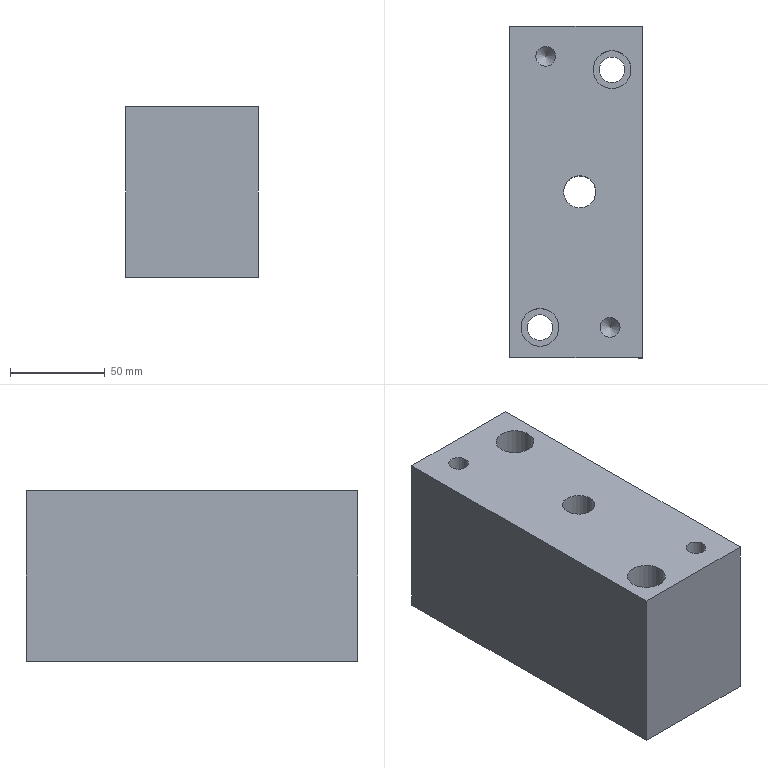Part | STEP file | lll_id4278_x_t | 1 solid | 17 faces | box 70 x 175 x 90 mm | volume 1031472 mm3 | plane 8 | cylinder 7 | cone 2 | commonest cylinder face diameters 10.506 x2 13.509 x2 20.008 x2 17 x1
STEP:
#1=CARTESIAN_POINT('',(3003.,-87.5,-90.));
#2=VERTEX_POINT('',#1);
#3=CARTESIAN_POINT('',(2933.,-87.5,-90.));
#4=VERTEX_POINT('',#3);
#5=CARTESIAN_POINT('',(13471.883,-87.5,-90.));
#6=DIRECTION('',(-1.,0.,0.));
#7=VECTOR('',#6,1.);
#8=LINE('',#5,#7);
#9=EDGE_CURVE('',#2,#4,#8,.T.);
#10=ORIENTED_EDGE('',*,*,#9,.F.);
#11=CARTESIAN_POINT('',(3003.,-87.5,0.));
#12=VERTEX_POINT('',#11);
#13=CARTESIAN_POINT('',(3003.,-87.5,0.));
#14=DIRECTION('',(0.,0.,1.));
#15=VECTOR('',#14,1.);
#16=LINE('',#13,#15);
#17=EDGE_CURVE('',#2,#12,#16,.T.);
#18=ORIENTED_EDGE('',*,*,#17,.T.);
#19=CARTESIAN_POINT('',(2933.,-87.5,0.));
#20=VERTEX_POINT('',#19);
#21=CARTESIAN_POINT('',(13471.883,-87.5,0.));
#22=DIRECTION('',(1.,0.,0.));
#23=VECTOR('',#22,1.);
#24=LINE('',#21,#23);
#25=EDGE_CURVE('',#20,#12,#24,.T.);
#26=ORIENTED_EDGE('',*,*,#25,.F.);
#27=CARTESIAN_POINT('',(2933.,-87.5,0.));
#28=DIRECTION('',(0.,0.,-1.));
#29=VECTOR('',#28,1.);
#30=LINE('',#27,#29);
#31=EDGE_CURVE('',#20,#4,#30,.T.);
#32=ORIENTED_EDGE('',*,*,#31,.T.);
#33=EDGE_LOOP('',(#10,#18,#26,#32));
#34=FACE_OUTER_BOUND('',#33,.T.);
#35=CARTESIAN_POINT('',(13471.883,-87.5,0.));
#36=DIRECTION('',(0.,1.,0.));
#37=DIRECTION('',(1.,0.,0.));
#38=AXIS2_PLACEMENT_3D('',#35,#36,#37);
#39=PLANE('',#38);
#40=ADVANCED_FACE('',(#34),#39,.F.);
#41=CARTESIAN_POINT('',(2933.,87.5,-90.));
#42=VERTEX_POINT('',#41);
#43=CARTESIAN_POINT('',(2933.,38.,-90.));
#44=DIRECTION('',(0.,-1.,0.));
#45=VECTOR('',#44,1.);
#46=LINE('',#43,#45);
#47=EDGE_CURVE('',#42,#4,#46,.T.);
#48=ORIENTED_EDGE('',*,*,#47,.T.);
#49=ORIENTED_EDGE('',*,*,#31,.F.);
#50=CARTESIAN_POINT('',(2933.,87.5,0.));
#51=VERTEX_POINT('',#50);
#52=CARTESIAN_POINT('',(2933.,38.,0.));
#53=DIRECTION('',(0.,-1.,0.));
#54=VECTOR('',#53,1.);
#55=LINE('',#52,#54);
#56=EDGE_CURVE('',#51,#20,#55,.T.);
#57=ORIENTED_EDGE('',*,*,#56,.F.);
#58=CARTESIAN_POINT('',(2933.,87.5,0.));
#59=DIRECTION('',(0.,0.,1.));
#60=VECTOR('',#59,1.);
#61=LINE('',#58,#60);
#62=EDGE_CURVE('',#42,#51,#61,.T.);
#63=ORIENTED_EDGE('',*,*,#62,.F.);
#64=EDGE_LOOP('',(#48,#49,#57,#63));
#65=FACE_OUTER_BOUND('',#64,.T.);
#66=CARTESIAN_POINT('',(2933.,38.,0.));
#67=DIRECTION('',(1.,0.,0.));
#68=DIRECTION('',(0.,-1.,0.));
#69=AXIS2_PLACEMENT_3D('',#66,#67,#68);
#70=PLANE('',#69);
#71=ADVANCED_FACE('',(#65),#70,.F.);
#72=CARTESIAN_POINT('',(3003.,87.5,-90.));
#73=VERTEX_POINT('',#72);
#74=CARTESIAN_POINT('',(13471.883,87.5,-90.));
#75=DIRECTION('',(1.,0.,0.));
#76=VECTOR('',#75,1.);
#77=LINE('',#74,#76);
#78=EDGE_CURVE('',#42,#73,#77,.T.);
#79=ORIENTED_EDGE('',*,*,#78,.F.);
#80=ORIENTED_EDGE('',*,*,#62,.T.);
#81=CARTESIAN_POINT('',(3003.,87.5,0.));
#82=VERTEX_POINT('',#81);
#83=CARTESIAN_POINT('',(13471.883,87.5,0.));
#84=DIRECTION('',(-1.,0.,0.));
#85=VECTOR('',#84,1.);
#86=LINE('',#83,#85);
#87=EDGE_CURVE('',#82,#51,#86,.T.);
#88=ORIENTED_EDGE('',*,*,#87,.F.);
#89=CARTESIAN_POINT('',(3003.,87.5,0.));
#90=DIRECTION('',(0.,0.,-1.));
#91=VECTOR('',#90,1.);
#92=LINE('',#89,#91);
#93=EDGE_CURVE('',#82,#73,#92,.T.);
#94=ORIENTED_EDGE('',*,*,#93,.T.);
#95=EDGE_LOOP('',(#79,#80,#88,#94));
#96=FACE_OUTER_BOUND('',#95,.T.);
#97=CARTESIAN_POINT('',(13471.883,87.5,0.));
#98=DIRECTION('',(0.,-1.,0.));
#99=DIRECTION('',(-1.,0.,0.));
#100=AXIS2_PLACEMENT_3D('',#97,#98,#99);
#101=PLANE('',#100);
#102=ADVANCED_FACE('',(#96),#101,.F.);
#103=CARTESIAN_POINT('',(3003.,-13712.786,-90.));
#104=DIRECTION('',(0.,-1.,0.));
#105=VECTOR('',#104,1.);
#106=LINE('',#103,#105);
#107=EDGE_CURVE('',#73,#2,#106,.T.);
#108=ORIENTED_EDGE('',*,*,#107,.F.);
#109=ORIENTED_EDGE('',*,*,#93,.F.);
#110=CARTESIAN_POINT('',(3003.,-13712.786,0.));
#111=DIRECTION('',(0.,1.,0.));
#112=VECTOR('',#111,1.);
#113=LINE('',#110,#112);
#114=EDGE_CURVE('',#12,#82,#113,.T.);
#115=ORIENTED_EDGE('',*,*,#114,.F.);
#116=ORIENTED_EDGE('',*,*,#17,.F.);
#117=EDGE_LOOP('',(#108,#109,#115,#116));
#118=FACE_OUTER_BOUND('',#117,.T.);
#119=CARTESIAN_POINT('',(3003.,-13712.786,0.));
#120=DIRECTION('',(-1.,0.,0.));
#121=DIRECTION('',(0.,1.,0.));
#122=AXIS2_PLACEMENT_3D('',#119,#120,#121);
#123=PLANE('',#122);
#124=ADVANCED_FACE('',(#118),#123,.F.);
#125=CARTESIAN_POINT('',(2978.5,0.,-90.));
#126=VERTEX_POINT('',#125);
#127=CARTESIAN_POINT('',(2970.,0.,-90.));
#128=DIRECTION('',(0.,0.,1.));
#129=DIRECTION('',(1.,0.,0.));
#130=AXIS2_PLACEMENT_3D('',#127,#128,#129);
#131=CIRCLE('',#130,8.5);
#132=EDGE_CURVE('',#126,#126,#131,.T.);
#133=ORIENTED_EDGE('',*,*,#132,.F.);
#134=EDGE_LOOP('',(#133));
#135=FACE_BOUND('',#134,.T.);
#136=CARTESIAN_POINT('',(2961.5,0.,0.));
#137=VERTEX_POINT('',#136);
#138=CARTESIAN_POINT('',(2970.,0.,0.));
#139=DIRECTION('',(0.,0.,1.));
#140=DIRECTION('',(-1.,0.,0.));
#141=AXIS2_PLACEMENT_3D('',#138,#139,#140);
#142=CIRCLE('',#141,8.5);
#143=EDGE_CURVE('',#137,#137,#142,.T.);
#144=ORIENTED_EDGE('',*,*,#143,.T.);
#145=EDGE_LOOP('',(#144));
#146=FACE_BOUND('',#145,.T.);
#147=CARTESIAN_POINT('',(2970.,0.,0.));
#148=DIRECTION('',(0.,0.,1.));
#149=DIRECTION('',(1.,0.,0.));
#150=AXIS2_PLACEMENT_3D('',#147,#148,#149);
#151=CYLINDRICAL_SURFACE('',#150,8.5);
#152=ADVANCED_FACE('',(#135,#146),#151,.F.);
#153=CARTESIAN_POINT('',(2997.004,64.5,0.));
#154=VERTEX_POINT('',#153);
#155=CARTESIAN_POINT('',(2987.,64.5,0.));
#156=DIRECTION('',(0.,0.,-1.));
#157=DIRECTION('',(1.,0.,0.));
#158=AXIS2_PLACEMENT_3D('',#155,#156,#157);
#159=CIRCLE('',#158,10.004);
#160=EDGE_CURVE('',#154,#154,#159,.T.);
#161=ORIENTED_EDGE('',*,*,#160,.T.);
#162=EDGE_LOOP('',(#161));
#163=FACE_BOUND('',#162,.T.);
#164=CARTESIAN_POINT('',(2946.747,71.5,0.));
#165=VERTEX_POINT('',#164);
#166=CARTESIAN_POINT('',(2952.,71.5,0.));
#167=DIRECTION('',(0.,0.,-1.));
#168=DIRECTION('',(-1.,0.,0.));
#169=AXIS2_PLACEMENT_3D('',#166,#167,#168);
#170=CIRCLE('',#169,5.253);
#171=EDGE_CURVE('',#165,#165,#170,.T.);
#172=ORIENTED_EDGE('',*,*,#171,.T.);
#173=EDGE_LOOP('',(#172));
#174=FACE_BOUND('',#173,.T.);
#175=CARTESIAN_POINT('',(2959.004,-71.5,0.));
#176=VERTEX_POINT('',#175);
#177=CARTESIAN_POINT('',(2949.,-71.5,0.));
#178=DIRECTION('',(0.,0.,-1.));
#179=DIRECTION('',(1.,0.,0.));
#180=AXIS2_PLACEMENT_3D('',#177,#178,#179);
#181=CIRCLE('',#180,10.004);
#182=EDGE_CURVE('',#176,#176,#181,.T.);
#183=ORIENTED_EDGE('',*,*,#182,.T.);
#184=EDGE_LOOP('',(#183));
#185=FACE_BOUND('',#184,.T.);
#186=CARTESIAN_POINT('',(2980.747,-71.5,0.));
#187=VERTEX_POINT('',#186);
#188=CARTESIAN_POINT('',(2986.,-71.5,0.));
#189=DIRECTION('',(0.,0.,-1.));
#190=DIRECTION('',(-1.,0.,0.));
#191=AXIS2_PLACEMENT_3D('',#188,#189,#190);
#192=CIRCLE('',#191,5.253);
#193=EDGE_CURVE('',#187,#187,#192,.T.);
#194=ORIENTED_EDGE('',*,*,#193,.T.);
#195=EDGE_LOOP('',(#194));
#196=FACE_BOUND('',#195,.T.);
#197=ORIENTED_EDGE('',*,*,#114,.T.);
#198=ORIENTED_EDGE('',*,*,#87,.T.);
#199=ORIENTED_EDGE('',*,*,#56,.T.);
#200=ORIENTED_EDGE('',*,*,#25,.T.);
#201=EDGE_LOOP('',(#197,#198,#199,#200));
#202=FACE_BOUND('',#201,.T.);
#203=ORIENTED_EDGE('',*,*,#143,.F.);
#204=EDGE_LOOP('',(#203));
#205=FACE_BOUND('',#204,.T.);
#206=CARTESIAN_POINT('',(13471.883,-13712.786,0.));
#207=DIRECTION('',(0.,0.,-1.));
#208=DIRECTION('',(-1.,0.,0.));
#209=AXIS2_PLACEMENT_3D('',#206,#207,#208);
#210=PLANE('',#209);
#211=ADVANCED_FACE('',(#163,#174,#185,#196,#202,#205),#210,.F.);
#212=CARTESIAN_POINT('',(2993.755,64.5,-90.));
#213=VERTEX_POINT('',#212);
#214=CARTESIAN_POINT('',(2987.,64.5,-90.));
#215=DIRECTION('',(0.,0.,1.));
#216=DIRECTION('',(1.,0.,0.));
#217=AXIS2_PLACEMENT_3D('',#214,#215,#216);
#218=CIRCLE('',#217,6.755);
#219=EDGE_CURVE('',#213,#213,#218,.T.);
#220=ORIENTED_EDGE('',*,*,#219,.T.);
#221=EDGE_LOOP('',(#220));
#222=FACE_BOUND('',#221,.T.);
#223=CARTESIAN_POINT('',(2955.755,-71.5,-90.));
#224=VERTEX_POINT('',#223);
#225=CARTESIAN_POINT('',(2949.,-71.5,-90.));
#226=DIRECTION('',(0.,0.,1.));
#227=DIRECTION('',(1.,0.,0.));
#228=AXIS2_PLACEMENT_3D('',#225,#226,#227);
#229=CIRCLE('',#228,6.755);
#230=EDGE_CURVE('',#224,#224,#229,.T.);
#231=ORIENTED_EDGE('',*,*,#230,.T.);
#232=EDGE_LOOP('',(#231));
#233=FACE_BOUND('',#232,.T.);
#234=ORIENTED_EDGE('',*,*,#9,.T.);
#235=ORIENTED_EDGE('',*,*,#47,.F.);
#236=ORIENTED_EDGE('',*,*,#78,.T.);
#237=ORIENTED_EDGE('',*,*,#107,.T.);
#238=EDGE_LOOP('',(#234,#235,#236,#237));
#239=FACE_BOUND('',#238,.T.);
#240=ORIENTED_EDGE('',*,*,#132,.T.);
#241=EDGE_LOOP('',(#240));
#242=FACE_BOUND('',#241,.T.);
#243=CARTESIAN_POINT('',(2968.,0.00007614,-90.));
#244=DIRECTION('',(0.,0.,1.));
#245=DIRECTION('',(1.,0.,0.));
#246=AXIS2_PLACEMENT_3D('',#243,#244,#245);
#247=PLANE('',#246);
#248=ADVANCED_FACE('',(#222,#233,#239,#242),#247,.F.);
#249=CARTESIAN_POINT('',(2980.747,-71.5,-32.753));
#250=VERTEX_POINT('',#249);
#251=CARTESIAN_POINT('',(2986.,-71.5,-32.753));
#252=DIRECTION('',(0.,0.,-1.));
#253=DIRECTION('',(-1.,0.,0.));
#254=AXIS2_PLACEMENT_3D('',#251,#252,#253);
#255=CIRCLE('',#254,5.253);
#256=EDGE_CURVE('',#250,#250,#255,.T.);
#257=ORIENTED_EDGE('',*,*,#256,.T.);
#258=EDGE_LOOP('',(#257));
#259=FACE_BOUND('',#258,.T.);
#260=ORIENTED_EDGE('',*,*,#193,.F.);
#261=EDGE_LOOP('',(#260));
#262=FACE_BOUND('',#261,.T.);
#263=CARTESIAN_POINT('',(2986.,-71.5,2.));
#264=DIRECTION('',(0.,0.,-1.));
#265=DIRECTION('',(1.,0.,0.));
#266=AXIS2_PLACEMENT_3D('',#263,#264,#265);
#267=CYLINDRICAL_SURFACE('',#266,5.253);
#268=ADVANCED_FACE('',(#259,#262),#267,.F.);
#269=CARTESIAN_POINT('',(2986.,-71.5,-38.006));
#270=VERTEX_POINT('',#269);
#271=VERTEX_LOOP('',#270);
#272=FACE_BOUND('',#271,.T.);
#273=ORIENTED_EDGE('',*,*,#256,.F.);
#274=EDGE_LOOP('',(#273));
#275=FACE_BOUND('',#274,.T.);
#276=CARTESIAN_POINT('',(2986.,-71.5,-32.753));
#277=DIRECTION('',(0.,0.,1.));
#278=DIRECTION('',(1.,0.,0.));
#279=AXIS2_PLACEMENT_3D('',#276,#277,#278);
#280=CONICAL_SURFACE('',#279,5.253,45.);
#281=ADVANCED_FACE('',(#272,#275),#280,.F.);
#282=CARTESIAN_POINT('',(2942.245,-71.5,-55.));
#283=VERTEX_POINT('',#282);
#284=CARTESIAN_POINT('',(2949.,-71.5,-55.));
#285=DIRECTION('',(0.,0.,-1.));
#286=DIRECTION('',(-1.,0.,0.));
#287=AXIS2_PLACEMENT_3D('',#284,#285,#286);
#288=CIRCLE('',#287,6.755);
#289=EDGE_CURVE('',#283,#283,#288,.T.);
#290=ORIENTED_EDGE('',*,*,#289,.F.);
#291=EDGE_LOOP('',(#290));
#292=FACE_BOUND('',#291,.T.);
#293=ORIENTED_EDGE('',*,*,#230,.F.);
#294=EDGE_LOOP('',(#293));
#295=FACE_BOUND('',#294,.T.);
#296=CARTESIAN_POINT('',(2949.,-71.5,2.));
#297=DIRECTION('',(0.,0.,-1.));
#298=DIRECTION('',(1.,0.,0.));
#299=AXIS2_PLACEMENT_3D('',#296,#297,#298);
#300=CYLINDRICAL_SURFACE('',#299,6.755);
#301=ADVANCED_FACE('',(#292,#295),#300,.F.);
#302=ORIENTED_EDGE('',*,*,#289,.T.);
#303=EDGE_LOOP('',(#302));
#304=FACE_BOUND('',#303,.T.);
#305=CARTESIAN_POINT('',(2959.004,-71.5,-55.));
#306=VERTEX_POINT('',#305);
#307=CARTESIAN_POINT('',(2949.,-71.5,-55.));
#308=DIRECTION('',(0.,0.,-1.));
#309=DIRECTION('',(1.,0.,0.));
#310=AXIS2_PLACEMENT_3D('',#307,#308,#309);
#311=CIRCLE('',#310,10.004);
#312=EDGE_CURVE('',#306,#306,#311,.T.);
#313=ORIENTED_EDGE('',*,*,#312,.F.);
#314=EDGE_LOOP('',(#313));
#315=FACE_BOUND('',#314,.T.);
#316=CARTESIAN_POINT('',(2949.,-71.5,-55.));
#317=DIRECTION('',(0.,0.,-1.));
#318=DIRECTION('',(-1.,0.,0.));
#319=AXIS2_PLACEMENT_3D('',#316,#317,#318);
#320=PLANE('',#319);
#321=ADVANCED_FACE('',(#304,#315),#320,.F.);
#322=ORIENTED_EDGE('',*,*,#312,.T.);
#323=EDGE_LOOP('',(#322));
#324=FACE_BOUND('',#323,.T.);
#325=ORIENTED_EDGE('',*,*,#182,.F.);
#326=EDGE_LOOP('',(#325));
#327=FACE_BOUND('',#326,.T.);
#328=CARTESIAN_POINT('',(2949.,-71.5,0.));
#329=DIRECTION('',(0.,0.,-1.));
#330=DIRECTION('',(1.,0.,0.));
#331=AXIS2_PLACEMENT_3D('',#328,#329,#330);
#332=CYLINDRICAL_SURFACE('',#331,10.004);
#333=ADVANCED_FACE('',(#324,#327),#332,.F.);
#334=CARTESIAN_POINT('',(2946.747,71.5,-32.753));
#335=VERTEX_POINT('',#334);
#336=CARTESIAN_POINT('',(2952.,71.5,-32.753));
#337=DIRECTION('',(0.,0.,-1.));
#338=DIRECTION('',(-1.,0.,0.));
#339=AXIS2_PLACEMENT_3D('',#336,#337,#338);
#340=CIRCLE('',#339,5.253);
#341=EDGE_CURVE('',#335,#335,#340,.T.);
#342=ORIENTED_EDGE('',*,*,#341,.T.);
#343=EDGE_LOOP('',(#342));
#344=FACE_BOUND('',#343,.T.);
#345=ORIENTED_EDGE('',*,*,#171,.F.);
#346=EDGE_LOOP('',(#345));
#347=FACE_BOUND('',#346,.T.);
#348=CARTESIAN_POINT('',(2952.,71.5,2.));
#349=DIRECTION('',(0.,0.,-1.));
#350=DIRECTION('',(1.,0.,0.));
#351=AXIS2_PLACEMENT_3D('',#348,#349,#350);
#352=CYLINDRICAL_SURFACE('',#351,5.253);
#353=ADVANCED_FACE('',(#344,#347),#352,.F.);
#354=CARTESIAN_POINT('',(2952.,71.5,-38.006));
#355=VERTEX_POINT('',#354);
#356=VERTEX_LOOP('',#355);
#357=FACE_BOUND('',#356,.T.);
#358=ORIENTED_EDGE('',*,*,#341,.F.);
#359=EDGE_LOOP('',(#358));
#360=FACE_BOUND('',#359,.T.);
#361=CARTESIAN_POINT('',(2952.,71.5,-32.753));
#362=DIRECTION('',(0.,0.,1.));
#363=DIRECTION('',(1.,0.,0.));
#364=AXIS2_PLACEMENT_3D('',#361,#362,#363);
#365=CONICAL_SURFACE('',#364,5.253,45.);
#366=ADVANCED_FACE('',(#357,#360),#365,.F.);
#367=CARTESIAN_POINT('',(2980.245,64.5,-55.));
#368=VERTEX_POINT('',#367);
#369=CARTESIAN_POINT('',(2987.,64.5,-55.));
#370=DIRECTION('',(0.,0.,-1.));
#371=DIRECTION('',(-1.,0.,0.));
#372=AXIS2_PLACEMENT_3D('',#369,#370,#371);
#373=CIRCLE('',#372,6.755);
#374=EDGE_CURVE('',#368,#368,#373,.T.);
#375=ORIENTED_EDGE('',*,*,#374,.F.);
#376=EDGE_LOOP('',(#375));
#377=FACE_BOUND('',#376,.T.);
#378=ORIENTED_EDGE('',*,*,#219,.F.);
#379=EDGE_LOOP('',(#378));
#380=FACE_BOUND('',#379,.T.);
#381=CARTESIAN_POINT('',(2987.,64.5,2.));
#382=DIRECTION('',(0.,0.,-1.));
#383=DIRECTION('',(1.,0.,0.));
#384=AXIS2_PLACEMENT_3D('',#381,#382,#383);
#385=CYLINDRICAL_SURFACE('',#384,6.755);
#386=ADVANCED_FACE('',(#377,#380),#385,.F.);
#387=ORIENTED_EDGE('',*,*,#374,.T.);
#388=EDGE_LOOP('',(#387));
#389=FACE_BOUND('',#388,.T.);
#390=CARTESIAN_POINT('',(2997.004,64.5,-55.));
#391=VERTEX_POINT('',#390);
#392=CARTESIAN_POINT('',(2987.,64.5,-55.));
#393=DIRECTION('',(0.,0.,-1.));
#394=DIRECTION('',(1.,0.,0.));
#395=AXIS2_PLACEMENT_3D('',#392,#393,#394);
#396=CIRCLE('',#395,10.004);
#397=EDGE_CURVE('',#391,#391,#396,.T.);
#398=ORIENTED_EDGE('',*,*,#397,.F.);
#399=EDGE_LOOP('',(#398));
#400=FACE_BOUND('',#399,.T.);
#401=CARTESIAN_POINT('',(2987.,64.5,-55.));
#402=DIRECTION('',(0.,0.,-1.));
#403=DIRECTION('',(-1.,0.,0.));
#404=AXIS2_PLACEMENT_3D('',#401,#402,#403);
#405=PLANE('',#404);
#406=ADVANCED_FACE('',(#389,#400),#405,.F.);
#407=ORIENTED_EDGE('',*,*,#397,.T.);
#408=EDGE_LOOP('',(#407));
#409=FACE_BOUND('',#408,.T.);
#410=ORIENTED_EDGE('',*,*,#160,.F.);
#411=EDGE_LOOP('',(#410));
#412=FACE_BOUND('',#411,.T.);
#413=CARTESIAN_POINT('',(2987.,64.5,0.));
#414=DIRECTION('',(0.,0.,-1.));
#415=DIRECTION('',(1.,0.,0.));
#416=AXIS2_PLACEMENT_3D('',#413,#414,#415);
#417=CYLINDRICAL_SURFACE('',#416,10.004);
#418=ADVANCED_FACE('',(#409,#412),#417,.F.);
#419=CLOSED_SHELL('',(#40,#71,#102,#124,#152,#211,#248,#268,#281,#301,#321,#333,#353,#366,#386,#406,#418));
#420=MANIFOLD_SOLID_BREP('',#419);
#421=(LENGTH_UNIT()NAMED_UNIT(*)SI_UNIT(.MILLI.,.METRE.));
#422=UNCERTAINTY_MEASURE_WITH_UNIT(LENGTH_MEASURE(0.00002),#421,'','');
#423=(NAMED_UNIT(*)PLANE_ANGLE_UNIT()SI_UNIT($,.RADIAN.));
#424=PLANE_ANGLE_MEASURE_WITH_UNIT(PLANE_ANGLE_MEASURE(0.01745),#423);
#425=DIMENSIONAL_EXPONENTS(0.,0.,0.,0.,0.,0.,0.);
#426=(CONVERSION_BASED_UNIT('DEGREE',#424)NAMED_UNIT(#425)PLANE_ANGLE_UNIT());
#427=(NAMED_UNIT(*)SI_UNIT($,.STERADIAN.)SOLID_ANGLE_UNIT());
#428=(GEOMETRIC_REPRESENTATION_CONTEXT(3)GLOBAL_UNCERTAINTY_ASSIGNED_CONTEXT((#422))GLOBAL_UNIT_ASSIGNED_CONTEXT((#421,#426,#427))REPRESENTATION_CONTEXT('',''));
#429=ADVANCED_BREP_SHAPE_REPRESENTATION('',(#420),#428);